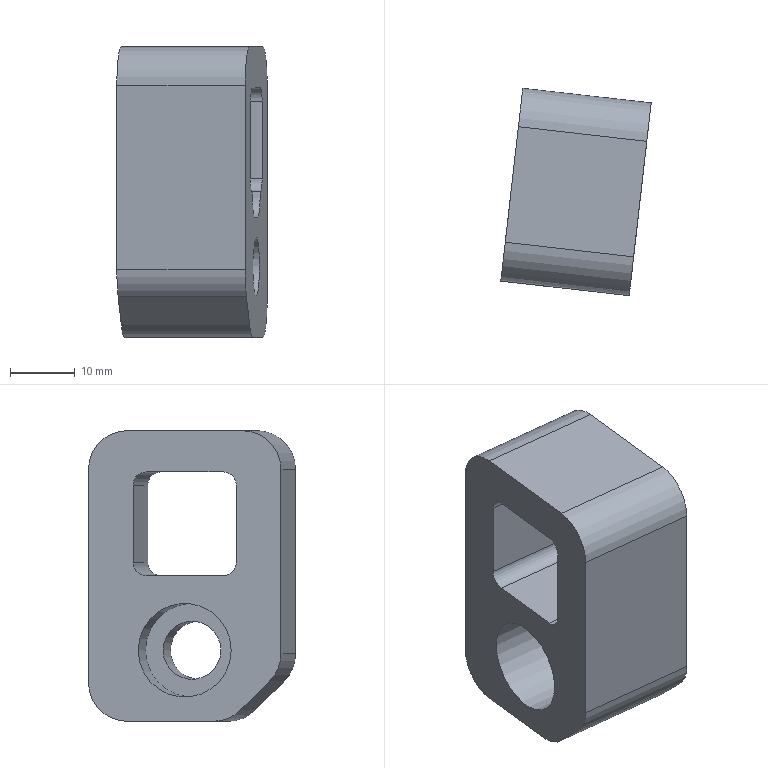Part | NX | features XQ 2 | 1 solid | 30 faces | box 23.268 x 32.071 x 45 mm | volume 18172 mm3 | plane 16 | cylinder 14 | commonest cylinder face diameters 12 x5 4.08 x4 8 x2 4 x1 9 x1 14.5 x1
STEP:
#1=CARTESIAN_POINT('',(3256.98,-253.634,-80.392));
#2=VERTEX_POINT('',#1);
#3=CARTESIAN_POINT('',(3257.49,-249.163,-80.392));
#4=DIRECTION('',(0.9936,-0.1132,0.));
#5=DIRECTION('',(-0.1132,-0.9936,0.));
#6=AXIS2_PLACEMENT_3D('',#3,#4,#5);
#7=CIRCLE('',#6,4.5);
#8=EDGE_CURVE('',#2,#2,#7,.T.);
#9=ORIENTED_EDGE('',*,*,#8,.F.);
#10=EDGE_LOOP('',(#9));
#11=FACE_BOUND('',#10,.T.);
#12=CARTESIAN_POINT('',(3259.188,-234.259,-85.392));
#13=VERTEX_POINT('',#12);
#14=CARTESIAN_POINT('',(3259.188,-234.259,-52.392));
#15=VERTEX_POINT('',#14);
#16=CARTESIAN_POINT('',(3259.188,-234.259,-78.616));
#17=DIRECTION('',(0.,0.,1.));
#18=VECTOR('',#17,1000.);
#19=LINE('',#16,#18);
#20=EDGE_CURVE('',#13,#15,#19,.T.);
#21=ORIENTED_EDGE('',*,*,#20,.T.);
#22=CARTESIAN_POINT('',(3258.508,-240.221,-46.392));
#23=VERTEX_POINT('',#22);
#24=CARTESIAN_POINT('',(3258.508,-240.221,-52.392));
#25=DIRECTION('',(0.9936,-0.1132,0.));
#26=DIRECTION('',(-0.1132,-0.9936,0.));
#27=AXIS2_PLACEMENT_3D('',#24,#25,#26);
#28=CIRCLE('',#27,6.);
#29=EDGE_CURVE('',#15,#23,#28,.T.);
#30=ORIENTED_EDGE('',*,*,#29,.T.);
#31=CARTESIAN_POINT('',(3256.471,-258.105,-46.392));
#32=VERTEX_POINT('',#31);
#33=CARTESIAN_POINT('',(3266.041,-174.108,-46.392));
#34=DIRECTION('',(-0.1132,-0.9936,0.));
#35=VECTOR('',#34,1000.);
#36=LINE('',#33,#35);
#37=EDGE_CURVE('',#23,#32,#36,.T.);
#38=ORIENTED_EDGE('',*,*,#37,.T.);
#39=CARTESIAN_POINT('',(3255.792,-264.066,-52.392));
#40=VERTEX_POINT('',#39);
#41=CARTESIAN_POINT('',(3256.471,-258.105,-52.392));
#42=DIRECTION('',(0.9936,-0.1132,0.));
#43=DIRECTION('',(-0.1132,-0.9936,0.));
#44=AXIS2_PLACEMENT_3D('',#41,#42,#43);
#45=CIRCLE('',#44,6.);
#46=EDGE_CURVE('',#32,#40,#45,.T.);
#47=ORIENTED_EDGE('',*,*,#46,.T.);
#48=CARTESIAN_POINT('',(3255.792,-264.066,-80.907));
#49=VERTEX_POINT('',#48);
#50=CARTESIAN_POINT('',(3255.792,-264.066,-78.616));
#51=DIRECTION('',(0.,0.,-1.));
#52=VECTOR('',#51,1000.);
#53=LINE('',#50,#52);
#54=EDGE_CURVE('',#40,#49,#53,.T.);
#55=ORIENTED_EDGE('',*,*,#54,.T.);
#56=CARTESIAN_POINT('',(3255.991,-262.32,-85.149));
#57=VERTEX_POINT('',#56);
#58=CARTESIAN_POINT('',(3256.471,-258.105,-80.907));
#59=DIRECTION('',(0.9936,-0.1132,0.));
#60=DIRECTION('',(-0.1132,-0.9936,0.));
#61=AXIS2_PLACEMENT_3D('',#58,#59,#60);
#62=CIRCLE('',#61,6.);
#63=EDGE_CURVE('',#49,#57,#62,.T.);
#64=ORIENTED_EDGE('',*,*,#63,.T.);
#65=CARTESIAN_POINT('',(3256.498,-257.864,-89.635));
#66=VERTEX_POINT('',#65);
#67=CARTESIAN_POINT('',(3260.646,-221.46,-126.274));
#68=DIRECTION('',(0.08005,0.7026,-0.7071));
#69=VECTOR('',#68,1000.);
#70=LINE('',#67,#69);
#71=EDGE_CURVE('',#57,#66,#70,.T.);
#72=ORIENTED_EDGE('',*,*,#71,.T.);
#73=CARTESIAN_POINT('',(3256.979,-253.648,-91.392));
#74=VERTEX_POINT('',#73);
#75=CARTESIAN_POINT('',(3256.979,-253.648,-85.392));
#76=DIRECTION('',(0.9936,-0.1132,0.));
#77=DIRECTION('',(-0.1132,-0.9936,0.));
#78=AXIS2_PLACEMENT_3D('',#75,#76,#77);
#79=CIRCLE('',#78,6.);
#80=EDGE_CURVE('',#66,#74,#79,.T.);
#81=ORIENTED_EDGE('',*,*,#80,.T.);
#82=CARTESIAN_POINT('',(3258.508,-240.221,-91.392));
#83=VERTEX_POINT('',#82);
#84=CARTESIAN_POINT('',(3266.041,-174.108,-91.392));
#85=DIRECTION('',(0.1132,0.9936,0.));
#86=VECTOR('',#85,1000.);
#87=LINE('',#84,#86);
#88=EDGE_CURVE('',#74,#83,#87,.T.);
#89=ORIENTED_EDGE('',*,*,#88,.T.);
#90=CARTESIAN_POINT('',(3258.508,-240.221,-85.392));
#91=DIRECTION('',(0.9936,-0.1132,0.));
#92=DIRECTION('',(-0.1132,-0.9936,0.));
#93=AXIS2_PLACEMENT_3D('',#90,#91,#92);
#94=CIRCLE('',#93,6.);
#95=EDGE_CURVE('',#83,#13,#94,.T.);
#96=ORIENTED_EDGE('',*,*,#95,.T.);
#97=EDGE_LOOP('',(#21,#30,#38,#47,#55,#64,#72,#81,#89,#96));
#98=FACE_BOUND('',#97,.T.);
#99=CARTESIAN_POINT('',(3257.32,-250.653,-72.892));
#100=VERTEX_POINT('',#99);
#101=CARTESIAN_POINT('',(3256.867,-254.627,-68.857));
#102=VERTEX_POINT('',#101);
#103=CARTESIAN_POINT('',(3257.32,-250.653,-68.892));
#104=DIRECTION('',(-0.9936,0.1132,0.));
#105=DIRECTION('',(-0.1132,-0.9936,0.));
#106=AXIS2_PLACEMENT_3D('',#103,#104,#105);
#107=CIRCLE('',#106,4.);
#108=EDGE_CURVE('',#100,#102,#107,.T.);
#109=ORIENTED_EDGE('',*,*,#108,.T.);
#110=CARTESIAN_POINT('',(3256.81,-255.124,-68.857));
#111=VERTEX_POINT('',#110);
#112=CARTESIAN_POINT('',(3258.112,-243.698,-68.857));
#113=DIRECTION('',(-0.1132,-0.9936,0.));
#114=VECTOR('',#113,1000.);
#115=LINE('',#112,#114);
#116=EDGE_CURVE('',#102,#111,#115,.T.);
#117=ORIENTED_EDGE('',*,*,#116,.T.);
#118=CARTESIAN_POINT('',(3256.579,-257.151,-66.817));
#119=VERTEX_POINT('',#118);
#120=CARTESIAN_POINT('',(3256.81,-255.124,-66.817));
#121=DIRECTION('',(-0.9936,0.1132,0.));
#122=DIRECTION('',(-0.1132,-0.9936,0.));
#123=AXIS2_PLACEMENT_3D('',#120,#121,#122);
#124=CIRCLE('',#123,2.04);
#125=EDGE_CURVE('',#111,#119,#124,.T.);
#126=ORIENTED_EDGE('',*,*,#125,.T.);
#127=CARTESIAN_POINT('',(3256.579,-257.151,-54.817));
#128=VERTEX_POINT('',#127);
#129=CARTESIAN_POINT('',(3256.579,-257.151,-66.817));
#130=DIRECTION('',(0.,-0.000000001,1.));
#131=VECTOR('',#130,1000.);
#132=LINE('',#129,#131);
#133=EDGE_CURVE('',#119,#128,#132,.T.);
#134=ORIENTED_EDGE('',*,*,#133,.T.);
#135=CARTESIAN_POINT('',(3256.81,-255.124,-52.777));
#136=VERTEX_POINT('',#135);
#137=CARTESIAN_POINT('',(3256.81,-255.124,-54.817));
#138=DIRECTION('',(-0.9936,0.1132,0.));
#139=DIRECTION('',(-0.1132,-0.9936,0.));
#140=AXIS2_PLACEMENT_3D('',#137,#138,#139);
#141=CIRCLE('',#140,2.04);
#142=EDGE_CURVE('',#128,#136,#141,.T.);
#143=ORIENTED_EDGE('',*,*,#142,.T.);
#144=CARTESIAN_POINT('',(3258.169,-243.201,-52.777));
#145=VERTEX_POINT('',#144);
#146=CARTESIAN_POINT('',(3256.81,-255.124,-52.777));
#147=DIRECTION('',(0.1132,0.9936,0.000000001));
#148=VECTOR('',#147,1000.);
#149=LINE('',#146,#148);
#150=EDGE_CURVE('',#136,#145,#149,.T.);
#151=ORIENTED_EDGE('',*,*,#150,.T.);
#152=CARTESIAN_POINT('',(3258.4,-241.174,-54.817));
#153=VERTEX_POINT('',#152);
#154=CARTESIAN_POINT('',(3258.169,-243.201,-54.817));
#155=DIRECTION('',(-0.9936,0.1132,0.));
#156=DIRECTION('',(-0.1132,-0.9936,0.));
#157=AXIS2_PLACEMENT_3D('',#154,#155,#156);
#158=CIRCLE('',#157,2.04);
#159=EDGE_CURVE('',#145,#153,#158,.T.);
#160=ORIENTED_EDGE('',*,*,#159,.T.);
#161=CARTESIAN_POINT('',(3258.4,-241.174,-66.817));
#162=VERTEX_POINT('',#161);
#163=CARTESIAN_POINT('',(3258.4,-241.174,-54.817));
#164=DIRECTION('',(0.,0.000000001,-1.));
#165=VECTOR('',#164,1000.);
#166=LINE('',#163,#165);
#167=EDGE_CURVE('',#153,#162,#166,.T.);
#168=ORIENTED_EDGE('',*,*,#167,.T.);
#169=CARTESIAN_POINT('',(3258.169,-243.201,-68.857));
#170=VERTEX_POINT('',#169);
#171=CARTESIAN_POINT('',(3258.169,-243.201,-66.817));
#172=DIRECTION('',(-0.9936,0.1132,0.));
#173=DIRECTION('',(-0.1132,-0.9936,0.));
#174=AXIS2_PLACEMENT_3D('',#171,#172,#173);
#175=CIRCLE('',#174,2.04);
#176=EDGE_CURVE('',#162,#170,#175,.T.);
#177=ORIENTED_EDGE('',*,*,#176,.T.);
#178=CARTESIAN_POINT('',(3258.112,-243.698,-68.857));
#179=VERTEX_POINT('',#178);
#180=CARTESIAN_POINT('',(3258.112,-243.698,-68.857));
#181=DIRECTION('',(-0.1132,-0.9936,0.));
#182=VECTOR('',#181,1000.);
#183=LINE('',#180,#182);
#184=EDGE_CURVE('',#170,#179,#183,.T.);
#185=ORIENTED_EDGE('',*,*,#184,.T.);
#186=CARTESIAN_POINT('',(3257.659,-247.672,-72.892));
#187=VERTEX_POINT('',#186);
#188=CARTESIAN_POINT('',(3257.659,-247.672,-68.892));
#189=DIRECTION('',(-0.9936,0.1132,0.));
#190=DIRECTION('',(-0.1132,-0.9936,0.));
#191=AXIS2_PLACEMENT_3D('',#188,#189,#190);
#192=CIRCLE('',#191,4.);
#193=EDGE_CURVE('',#179,#187,#192,.T.);
#194=ORIENTED_EDGE('',*,*,#193,.T.);
#195=CARTESIAN_POINT('',(3258.112,-243.698,-72.892));
#196=DIRECTION('',(-0.1132,-0.9936,0.));
#197=VECTOR('',#196,1000.);
#198=LINE('',#195,#197);
#199=EDGE_CURVE('',#187,#100,#198,.T.);
#200=ORIENTED_EDGE('',*,*,#199,.T.);
#201=EDGE_LOOP('',(#109,#117,#126,#134,#143,#151,#160,#168,#177,#185,#194,#200));
#202=FACE_BOUND('',#201,.T.);
#203=CARTESIAN_POINT('',(3266.041,-174.108,-78.616));
#204=DIRECTION('',(0.9936,-0.1132,0.));
#205=DIRECTION('',(-0.1132,-0.9936,0.));
#206=AXIS2_PLACEMENT_3D('',#203,#204,#205);
#207=PLANE('',#206);
#208=ADVANCED_FACE('',(#11,#98,#202),#207,.T.);
#209=CARTESIAN_POINT('',(3236.708,-254.887,-66.817));
#210=VERTEX_POINT('',#209);
#211=CARTESIAN_POINT('',(3236.708,-254.887,-54.817));
#212=VERTEX_POINT('',#211);
#213=CARTESIAN_POINT('',(3236.708,-254.887,-39.152));
#214=DIRECTION('',(0.,-0.000000001,1.));
#215=VECTOR('',#214,1000.);
#216=LINE('',#213,#215);
#217=EDGE_CURVE('',#210,#212,#216,.T.);
#218=ORIENTED_EDGE('',*,*,#217,.F.);
#219=CARTESIAN_POINT('',(3236.939,-252.86,-68.857));
#220=VERTEX_POINT('',#219);
#221=CARTESIAN_POINT('',(3236.939,-252.86,-66.817));
#222=DIRECTION('',(-0.9936,0.1132,0.));
#223=DIRECTION('',(0.1132,0.9936,0.));
#224=AXIS2_PLACEMENT_3D('',#221,#222,#223);
#225=CIRCLE('',#224,2.04);
#226=EDGE_CURVE('',#220,#210,#225,.T.);
#227=ORIENTED_EDGE('',*,*,#226,.F.);
#228=CARTESIAN_POINT('',(3238.297,-240.937,-68.857));
#229=VERTEX_POINT('',#228);
#230=CARTESIAN_POINT('',(3256.924,-77.454,-68.857));
#231=DIRECTION('',(-0.1132,-0.9936,0.));
#232=VECTOR('',#231,1000.);
#233=LINE('',#230,#232);
#234=EDGE_CURVE('',#229,#220,#233,.T.);
#235=ORIENTED_EDGE('',*,*,#234,.F.);
#236=CARTESIAN_POINT('',(3238.528,-238.91,-66.817));
#237=VERTEX_POINT('',#236);
#238=CARTESIAN_POINT('',(3238.297,-240.937,-66.817));
#239=DIRECTION('',(-0.9936,0.1132,0.));
#240=DIRECTION('',(0.1132,0.9936,0.));
#241=AXIS2_PLACEMENT_3D('',#238,#239,#240);
#242=CIRCLE('',#241,2.04);
#243=EDGE_CURVE('',#237,#229,#242,.T.);
#244=ORIENTED_EDGE('',*,*,#243,.F.);
#245=CARTESIAN_POINT('',(3238.528,-238.91,-54.817));
#246=VERTEX_POINT('',#245);
#247=CARTESIAN_POINT('',(3238.528,-238.91,-39.152));
#248=DIRECTION('',(0.,0.000000001,-1.));
#249=VECTOR('',#248,1000.);
#250=LINE('',#247,#249);
#251=EDGE_CURVE('',#246,#237,#250,.T.);
#252=ORIENTED_EDGE('',*,*,#251,.F.);
#253=CARTESIAN_POINT('',(3238.297,-240.937,-52.777));
#254=VERTEX_POINT('',#253);
#255=CARTESIAN_POINT('',(3238.297,-240.937,-54.817));
#256=DIRECTION('',(-0.9936,0.1132,0.));
#257=DIRECTION('',(0.1132,0.9936,0.));
#258=AXIS2_PLACEMENT_3D('',#255,#256,#257);
#259=CIRCLE('',#258,2.04);
#260=EDGE_CURVE('',#254,#246,#259,.T.);
#261=ORIENTED_EDGE('',*,*,#260,.F.);
#262=CARTESIAN_POINT('',(3236.939,-252.86,-52.777));
#263=VERTEX_POINT('',#262);
#264=CARTESIAN_POINT('',(3256.924,-77.454,-52.777));
#265=DIRECTION('',(0.1132,0.9936,0.000000001));
#266=VECTOR('',#265,1000.);
#267=LINE('',#264,#266);
#268=EDGE_CURVE('',#263,#254,#267,.T.);
#269=ORIENTED_EDGE('',*,*,#268,.F.);
#270=CARTESIAN_POINT('',(3236.939,-252.86,-54.817));
#271=DIRECTION('',(-0.9936,0.1132,0.));
#272=DIRECTION('',(0.1132,0.9936,0.));
#273=AXIS2_PLACEMENT_3D('',#270,#271,#272);
#274=CIRCLE('',#273,2.04);
#275=EDGE_CURVE('',#212,#263,#274,.T.);
#276=ORIENTED_EDGE('',*,*,#275,.F.);
#277=EDGE_LOOP('',(#218,#227,#235,#244,#252,#261,#269,#276));
#278=FACE_BOUND('',#277,.T.);
#279=CARTESIAN_POINT('',(3236.599,-255.841,-46.392));
#280=VERTEX_POINT('',#279);
#281=CARTESIAN_POINT('',(3238.637,-237.957,-46.392));
#282=VERTEX_POINT('',#281);
#283=CARTESIAN_POINT('',(3256.924,-77.454,-46.392));
#284=DIRECTION('',(0.1132,0.9936,0.));
#285=VECTOR('',#284,1000.);
#286=LINE('',#283,#285);
#287=EDGE_CURVE('',#280,#282,#286,.T.);
#288=ORIENTED_EDGE('',*,*,#287,.T.);
#289=CARTESIAN_POINT('',(3239.316,-231.995,-52.392));
#290=VERTEX_POINT('',#289);
#291=CARTESIAN_POINT('',(3238.637,-237.957,-52.392));
#292=DIRECTION('',(-0.9936,0.1132,0.));
#293=DIRECTION('',(0.1132,0.9936,0.));
#294=AXIS2_PLACEMENT_3D('',#291,#292,#293);
#295=CIRCLE('',#294,6.);
#296=EDGE_CURVE('',#282,#290,#295,.T.);
#297=ORIENTED_EDGE('',*,*,#296,.T.);
#298=CARTESIAN_POINT('',(3239.316,-231.995,-85.392));
#299=VERTEX_POINT('',#298);
#300=CARTESIAN_POINT('',(3239.316,-231.995,-39.152));
#301=DIRECTION('',(0.,0.,-1.));
#302=VECTOR('',#301,1000.);
#303=LINE('',#300,#302);
#304=EDGE_CURVE('',#290,#299,#303,.T.);
#305=ORIENTED_EDGE('',*,*,#304,.T.);
#306=CARTESIAN_POINT('',(3238.637,-237.957,-91.392));
#307=VERTEX_POINT('',#306);
#308=CARTESIAN_POINT('',(3238.637,-237.957,-85.392));
#309=DIRECTION('',(-0.9936,0.1132,0.));
#310=DIRECTION('',(0.1132,0.9936,0.));
#311=AXIS2_PLACEMENT_3D('',#308,#309,#310);
#312=CIRCLE('',#311,6.);
#313=EDGE_CURVE('',#299,#307,#312,.T.);
#314=ORIENTED_EDGE('',*,*,#313,.T.);
#315=CARTESIAN_POINT('',(3237.107,-251.384,-91.392));
#316=VERTEX_POINT('',#315);
#317=CARTESIAN_POINT('',(3256.924,-77.454,-91.392));
#318=DIRECTION('',(-0.1132,-0.9936,0.));
#319=VECTOR('',#318,1000.);
#320=LINE('',#317,#319);
#321=EDGE_CURVE('',#307,#316,#320,.T.);
#322=ORIENTED_EDGE('',*,*,#321,.T.);
#323=CARTESIAN_POINT('',(3236.627,-255.6,-89.635));
#324=VERTEX_POINT('',#323);
#325=CARTESIAN_POINT('',(3237.107,-251.384,-85.392));
#326=DIRECTION('',(-0.9936,0.1132,0.));
#327=DIRECTION('',(0.1132,0.9936,0.));
#328=AXIS2_PLACEMENT_3D('',#325,#326,#327);
#329=CIRCLE('',#328,6.);
#330=EDGE_CURVE('',#316,#324,#329,.T.);
#331=ORIENTED_EDGE('',*,*,#330,.T.);
#332=CARTESIAN_POINT('',(3236.119,-260.056,-85.149));
#333=VERTEX_POINT('',#332);
#334=CARTESIAN_POINT('',(3243.918,-191.606,-154.042));
#335=DIRECTION('',(-0.08005,-0.7026,0.7071));
#336=VECTOR('',#335,1000.);
#337=LINE('',#334,#336);
#338=EDGE_CURVE('',#324,#333,#337,.T.);
#339=ORIENTED_EDGE('',*,*,#338,.T.);
#340=CARTESIAN_POINT('',(3235.92,-261.802,-80.907));
#341=VERTEX_POINT('',#340);
#342=CARTESIAN_POINT('',(3236.599,-255.841,-80.907));
#343=DIRECTION('',(-0.9936,0.1132,0.));
#344=DIRECTION('',(0.1132,0.9936,0.));
#345=AXIS2_PLACEMENT_3D('',#342,#343,#344);
#346=CIRCLE('',#345,6.);
#347=EDGE_CURVE('',#333,#341,#346,.T.);
#348=ORIENTED_EDGE('',*,*,#347,.T.);
#349=CARTESIAN_POINT('',(3235.92,-261.802,-52.392));
#350=VERTEX_POINT('',#349);
#351=CARTESIAN_POINT('',(3235.92,-261.802,-39.152));
#352=DIRECTION('',(0.,0.,1.));
#353=VECTOR('',#352,1000.);
#354=LINE('',#351,#353);
#355=EDGE_CURVE('',#341,#350,#354,.T.);
#356=ORIENTED_EDGE('',*,*,#355,.T.);
#357=CARTESIAN_POINT('',(3236.599,-255.841,-52.392));
#358=DIRECTION('',(-0.9936,0.1132,0.));
#359=DIRECTION('',(0.1132,0.9936,0.));
#360=AXIS2_PLACEMENT_3D('',#357,#358,#359);
#361=CIRCLE('',#360,6.);
#362=EDGE_CURVE('',#350,#280,#361,.T.);
#363=ORIENTED_EDGE('',*,*,#362,.T.);
#364=EDGE_LOOP('',(#288,#297,#305,#314,#322,#331,#339,#348,#356,#363));
#365=FACE_BOUND('',#364,.T.);
#366=CARTESIAN_POINT('',(3238.439,-239.695,-80.392));
#367=VERTEX_POINT('',#366);
#368=CARTESIAN_POINT('',(3237.618,-246.899,-80.392));
#369=DIRECTION('',(0.9936,-0.1132,0.));
#370=DIRECTION('',(0.1132,0.9936,0.));
#371=AXIS2_PLACEMENT_3D('',#368,#369,#370);
#372=CIRCLE('',#371,7.25);
#373=EDGE_CURVE('',#367,#367,#372,.T.);
#374=ORIENTED_EDGE('',*,*,#373,.T.);
#375=EDGE_LOOP('',(#374));
#376=FACE_BOUND('',#375,.T.);
#377=CARTESIAN_POINT('',(3256.924,-77.454,-39.152));
#378=DIRECTION('',(-0.9936,0.1132,0.));
#379=DIRECTION('',(0.,0.,-1.));
#380=AXIS2_PLACEMENT_3D('',#377,#378,#379);
#381=PLANE('',#380);
#382=ADVANCED_FACE('',(#278,#365,#376),#381,.T.);
#383=ORIENTED_EDGE('',*,*,#37,.F.);
#384=CARTESIAN_POINT('',(3233.669,-237.391,-46.392));
#385=DIRECTION('',(-0.9936,0.1132,0.));
#386=VECTOR('',#385,1000.);
#387=LINE('',#384,#386);
#388=EDGE_CURVE('',#23,#282,#387,.T.);
#389=ORIENTED_EDGE('',*,*,#388,.T.);
#390=ORIENTED_EDGE('',*,*,#287,.F.);
#391=CARTESIAN_POINT('',(3231.631,-255.275,-46.392));
#392=DIRECTION('',(0.9936,-0.1132,0.));
#393=VECTOR('',#392,1000.);
#394=LINE('',#391,#393);
#395=EDGE_CURVE('',#280,#32,#394,.T.);
#396=ORIENTED_EDGE('',*,*,#395,.T.);
#397=EDGE_LOOP('',(#383,#389,#390,#396));
#398=FACE_BOUND('',#397,.T.);
#399=CARTESIAN_POINT('',(3232.65,-246.333,-46.392));
#400=DIRECTION('',(0.,0.,1.));
#401=DIRECTION('',(-0.9981,-0.06105,0.));
#402=AXIS2_PLACEMENT_3D('',#399,#400,#401);
#403=PLANE('',#402);
#404=ADVANCED_FACE('',(#398),#403,.T.);
#405=ORIENTED_EDGE('',*,*,#304,.F.);
#406=CARTESIAN_POINT('',(3234.348,-231.429,-52.392));
#407=DIRECTION('',(0.9936,-0.1132,0.));
#408=VECTOR('',#407,1000.);
#409=LINE('',#406,#408);
#410=EDGE_CURVE('',#290,#15,#409,.T.);
#411=ORIENTED_EDGE('',*,*,#410,.T.);
#412=ORIENTED_EDGE('',*,*,#20,.F.);
#413=CARTESIAN_POINT('',(3234.348,-231.429,-85.392));
#414=DIRECTION('',(-0.9936,0.1132,0.));
#415=VECTOR('',#414,1000.);
#416=LINE('',#413,#415);
#417=EDGE_CURVE('',#13,#299,#416,.T.);
#418=ORIENTED_EDGE('',*,*,#417,.T.);
#419=EDGE_LOOP('',(#405,#411,#412,#418));
#420=FACE_BOUND('',#419,.T.);
#421=CARTESIAN_POINT('',(3234.348,-231.429,-60.817));
#422=DIRECTION('',(0.1132,0.9936,0.));
#423=DIRECTION('',(0.9936,-0.1132,0.));
#424=AXIS2_PLACEMENT_3D('',#421,#422,#423);
#425=PLANE('',#424);
#426=ADVANCED_FACE('',(#420),#425,.T.);
#427=ORIENTED_EDGE('',*,*,#54,.F.);
#428=CARTESIAN_POINT('',(3230.952,-261.236,-52.392));
#429=DIRECTION('',(-0.9936,0.1132,0.));
#430=VECTOR('',#429,1000.);
#431=LINE('',#428,#430);
#432=EDGE_CURVE('',#40,#350,#431,.T.);
#433=ORIENTED_EDGE('',*,*,#432,.T.);
#434=ORIENTED_EDGE('',*,*,#355,.F.);
#435=CARTESIAN_POINT('',(3230.952,-261.236,-80.907));
#436=DIRECTION('',(0.9936,-0.1132,0.));
#437=VECTOR('',#436,1000.);
#438=LINE('',#435,#437);
#439=EDGE_CURVE('',#341,#49,#438,.T.);
#440=ORIENTED_EDGE('',*,*,#439,.T.);
#441=EDGE_LOOP('',(#427,#433,#434,#440));
#442=FACE_BOUND('',#441,.T.);
#443=CARTESIAN_POINT('',(3230.952,-261.236,-60.817));
#444=DIRECTION('',(-0.1132,-0.9936,0.));
#445=DIRECTION('',(-0.9936,0.1132,0.));
#446=AXIS2_PLACEMENT_3D('',#443,#444,#445);
#447=PLANE('',#446);
#448=ADVANCED_FACE('',(#442),#447,.T.);
#449=ORIENTED_EDGE('',*,*,#88,.F.);
#450=CARTESIAN_POINT('',(3232.139,-250.818,-91.392));
#451=DIRECTION('',(-0.9936,0.1132,0.));
#452=VECTOR('',#451,1000.);
#453=LINE('',#450,#452);
#454=EDGE_CURVE('',#74,#316,#453,.T.);
#455=ORIENTED_EDGE('',*,*,#454,.T.);
#456=ORIENTED_EDGE('',*,*,#321,.F.);
#457=CARTESIAN_POINT('',(3233.669,-237.391,-91.392));
#458=DIRECTION('',(0.9936,-0.1132,0.));
#459=VECTOR('',#458,1000.);
#460=LINE('',#457,#459);
#461=EDGE_CURVE('',#307,#83,#460,.T.);
#462=ORIENTED_EDGE('',*,*,#461,.T.);
#463=EDGE_LOOP('',(#449,#455,#456,#462));
#464=FACE_BOUND('',#463,.T.);
#465=CARTESIAN_POINT('',(3232.65,-246.333,-91.392));
#466=DIRECTION('',(0.,0.,-1.));
#467=DIRECTION('',(0.9981,0.06105,0.));
#468=AXIS2_PLACEMENT_3D('',#465,#466,#467);
#469=PLANE('',#468);
#470=ADVANCED_FACE('',(#464),#469,.T.);
#471=ORIENTED_EDGE('',*,*,#71,.F.);
#472=CARTESIAN_POINT('',(3231.151,-259.49,-85.149));
#473=DIRECTION('',(-0.9936,0.1132,0.));
#474=VECTOR('',#473,1000.);
#475=LINE('',#472,#474);
#476=EDGE_CURVE('',#57,#333,#475,.T.);
#477=ORIENTED_EDGE('',*,*,#476,.T.);
#478=ORIENTED_EDGE('',*,*,#338,.F.);
#479=CARTESIAN_POINT('',(3231.659,-255.034,-89.635));
#480=DIRECTION('',(0.9936,-0.1132,0.));
#481=VECTOR('',#480,1000.);
#482=LINE('',#479,#481);
#483=EDGE_CURVE('',#324,#66,#482,.T.);
#484=ORIENTED_EDGE('',*,*,#483,.T.);
#485=EDGE_LOOP('',(#471,#477,#478,#484));
#486=FACE_BOUND('',#485,.T.);
#487=CARTESIAN_POINT('',(3231.179,-259.249,-85.392));
#488=DIRECTION('',(0.08005,0.7026,0.7071));
#489=DIRECTION('',(0.9936,-0.1132,0.));
#490=AXIS2_PLACEMENT_3D('',#487,#488,#489);
#491=PLANE('',#490);
#492=ADVANCED_FACE('',(#486),#491,.F.);
#493=ORIENTED_EDGE('',*,*,#296,.F.);
#494=ORIENTED_EDGE('',*,*,#388,.F.);
#495=ORIENTED_EDGE('',*,*,#29,.F.);
#496=ORIENTED_EDGE('',*,*,#410,.F.);
#497=EDGE_LOOP('',(#493,#494,#495,#496));
#498=FACE_BOUND('',#497,.T.);
#499=CARTESIAN_POINT('',(3233.669,-237.391,-52.392));
#500=DIRECTION('',(0.9936,-0.1132,0.));
#501=DIRECTION('',(-0.1132,-0.9936,0.));
#502=AXIS2_PLACEMENT_3D('',#499,#500,#501);
#503=CYLINDRICAL_SURFACE('',#502,6.);
#504=ADVANCED_FACE('',(#498),#503,.T.);
#505=ORIENTED_EDGE('',*,*,#46,.F.);
#506=ORIENTED_EDGE('',*,*,#395,.F.);
#507=ORIENTED_EDGE('',*,*,#362,.F.);
#508=ORIENTED_EDGE('',*,*,#432,.F.);
#509=EDGE_LOOP('',(#505,#506,#507,#508));
#510=FACE_BOUND('',#509,.T.);
#511=CARTESIAN_POINT('',(3231.631,-255.275,-52.392));
#512=DIRECTION('',(-0.9936,0.1132,0.));
#513=DIRECTION('',(0.1132,0.9936,0.));
#514=AXIS2_PLACEMENT_3D('',#511,#512,#513);
#515=CYLINDRICAL_SURFACE('',#514,6.);
#516=ADVANCED_FACE('',(#510),#515,.T.);
#517=ORIENTED_EDGE('',*,*,#347,.F.);
#518=ORIENTED_EDGE('',*,*,#476,.F.);
#519=ORIENTED_EDGE('',*,*,#63,.F.);
#520=ORIENTED_EDGE('',*,*,#439,.F.);
#521=EDGE_LOOP('',(#517,#518,#519,#520));
#522=FACE_BOUND('',#521,.T.);
#523=CARTESIAN_POINT('',(3231.631,-255.275,-80.907));
#524=DIRECTION('',(-0.9936,0.1132,0.));
#525=DIRECTION('',(0.1132,0.9936,0.));
#526=AXIS2_PLACEMENT_3D('',#523,#524,#525);
#527=CYLINDRICAL_SURFACE('',#526,6.);
#528=ADVANCED_FACE('',(#522),#527,.T.);
#529=ORIENTED_EDGE('',*,*,#80,.F.);
#530=ORIENTED_EDGE('',*,*,#483,.F.);
#531=ORIENTED_EDGE('',*,*,#330,.F.);
#532=ORIENTED_EDGE('',*,*,#454,.F.);
#533=EDGE_LOOP('',(#529,#530,#531,#532));
#534=FACE_BOUND('',#533,.T.);
#535=CARTESIAN_POINT('',(3232.139,-250.818,-85.392));
#536=DIRECTION('',(0.9936,-0.1132,0.));
#537=DIRECTION('',(-0.1132,-0.9936,0.));
#538=AXIS2_PLACEMENT_3D('',#535,#536,#537);
#539=CYLINDRICAL_SURFACE('',#538,6.);
#540=ADVANCED_FACE('',(#534),#539,.T.);
#541=ORIENTED_EDGE('',*,*,#313,.F.);
#542=ORIENTED_EDGE('',*,*,#417,.F.);
#543=ORIENTED_EDGE('',*,*,#95,.F.);
#544=ORIENTED_EDGE('',*,*,#461,.F.);
#545=EDGE_LOOP('',(#541,#542,#543,#544));
#546=FACE_BOUND('',#545,.T.);
#547=CARTESIAN_POINT('',(3233.669,-237.391,-85.392));
#548=DIRECTION('',(0.9936,-0.1132,0.));
#549=DIRECTION('',(-0.1132,-0.9936,0.));
#550=AXIS2_PLACEMENT_3D('',#547,#548,#549);
#551=CYLINDRICAL_SURFACE('',#550,6.);
#552=ADVANCED_FACE('',(#546),#551,.T.);
#553=ORIENTED_EDGE('',*,*,#8,.T.);
#554=EDGE_LOOP('',(#553));
#555=FACE_BOUND('',#554,.T.);
#556=CARTESIAN_POINT('',(3247.044,-252.502,-80.392));
#557=VERTEX_POINT('',#556);
#558=CARTESIAN_POINT('',(3247.554,-248.031,-80.392));
#559=DIRECTION('',(0.9936,-0.1132,0.));
#560=DIRECTION('',(-0.1132,-0.9936,0.));
#561=AXIS2_PLACEMENT_3D('',#558,#559,#560);
#562=CIRCLE('',#561,4.5);
#563=EDGE_CURVE('',#557,#557,#562,.T.);
#564=ORIENTED_EDGE('',*,*,#563,.F.);
#565=EDGE_LOOP('',(#564));
#566=FACE_BOUND('',#565,.T.);
#567=CARTESIAN_POINT('',(3232.65,-246.333,-80.392));
#568=DIRECTION('',(0.9936,-0.1132,0.));
#569=DIRECTION('',(0.01966,0.1725,0.9848));
#570=AXIS2_PLACEMENT_3D('',#567,#568,#569);
#571=CYLINDRICAL_SURFACE('',#570,4.5);
#572=ADVANCED_FACE('',(#555,#566),#571,.F.);
#573=ORIENTED_EDGE('',*,*,#563,.T.);
#574=EDGE_LOOP('',(#573));
#575=FACE_BOUND('',#574,.T.);
#576=CARTESIAN_POINT('',(3246.733,-255.234,-80.392));
#577=VERTEX_POINT('',#576);
#578=CARTESIAN_POINT('',(3247.554,-248.031,-80.392));
#579=DIRECTION('',(0.9936,-0.1132,0.));
#580=DIRECTION('',(-0.1132,-0.9936,0.));
#581=AXIS2_PLACEMENT_3D('',#578,#579,#580);
#582=CIRCLE('',#581,7.25);
#583=EDGE_CURVE('',#577,#577,#582,.T.);
#584=ORIENTED_EDGE('',*,*,#583,.F.);
#585=EDGE_LOOP('',(#584));
#586=FACE_BOUND('',#585,.T.);
#587=CARTESIAN_POINT('',(3247.554,-248.031,-80.392));
#588=DIRECTION('',(0.9936,-0.1132,0.));
#589=DIRECTION('',(-0.1132,-0.9936,0.));
#590=AXIS2_PLACEMENT_3D('',#587,#588,#589);
#591=PLANE('',#590);
#592=ADVANCED_FACE('',(#575,#586),#591,.F.);
#593=ORIENTED_EDGE('',*,*,#583,.T.);
#594=EDGE_LOOP('',(#593));
#595=FACE_BOUND('',#594,.T.);
#596=ORIENTED_EDGE('',*,*,#373,.F.);
#597=EDGE_LOOP('',(#596));
#598=FACE_BOUND('',#597,.T.);
#599=CARTESIAN_POINT('',(3232.65,-246.333,-80.392));
#600=DIRECTION('',(0.9936,-0.1132,0.));
#601=DIRECTION('',(0.01966,0.1725,0.9848));
#602=AXIS2_PLACEMENT_3D('',#599,#600,#601);
#603=CYLINDRICAL_SURFACE('',#602,7.25);
#604=ADVANCED_FACE('',(#595,#598),#603,.F.);
#605=ORIENTED_EDGE('',*,*,#199,.F.);
#606=CARTESIAN_POINT('',(3249.711,-246.767,-72.892));
#607=VERTEX_POINT('',#606);
#608=CARTESIAN_POINT('',(3249.711,-246.767,-72.892));
#609=DIRECTION('',(-0.9936,0.1132,0.));
#610=VECTOR('',#609,1000.);
#611=LINE('',#608,#610);
#612=EDGE_CURVE('',#187,#607,#611,.T.);
#613=ORIENTED_EDGE('',*,*,#612,.T.);
#614=CARTESIAN_POINT('',(3249.371,-249.747,-72.892));
#615=VERTEX_POINT('',#614);
#616=CARTESIAN_POINT('',(3250.164,-242.792,-72.892));
#617=DIRECTION('',(-0.1132,-0.9936,0.));
#618=VECTOR('',#617,1000.);
#619=LINE('',#616,#618);
#620=EDGE_CURVE('',#607,#615,#619,.T.);
#621=ORIENTED_EDGE('',*,*,#620,.T.);
#622=CARTESIAN_POINT('',(3257.32,-250.653,-72.892));
#623=DIRECTION('',(0.9936,-0.1132,0.));
#624=VECTOR('',#623,1000.);
#625=LINE('',#622,#624);
#626=EDGE_CURVE('',#615,#100,#625,.T.);
#627=ORIENTED_EDGE('',*,*,#626,.T.);
#628=EDGE_LOOP('',(#605,#613,#621,#627));
#629=FACE_BOUND('',#628,.T.);
#630=CARTESIAN_POINT('',(3297.855,-248.226,-72.892));
#631=DIRECTION('',(0.,0.,-1.));
#632=DIRECTION('',(0.06105,-0.9981,0.));
#633=AXIS2_PLACEMENT_3D('',#630,#631,#632);
#634=PLANE('',#633);
#635=ADVANCED_FACE('',(#629),#634,.F.);
#636=CARTESIAN_POINT('',(3248.918,-253.722,-68.857));
#637=VERTEX_POINT('',#636);
#638=CARTESIAN_POINT('',(3249.145,-251.735,-68.857));
#639=VERTEX_POINT('',#638);
#640=CARTESIAN_POINT('',(3258.092,-173.202,-68.857));
#641=DIRECTION('',(0.1132,0.9936,0.));
#642=VECTOR('',#641,1000.);
#643=LINE('',#640,#642);
#644=EDGE_CURVE('',#637,#639,#643,.T.);
#645=ORIENTED_EDGE('',*,*,#644,.F.);
#646=CARTESIAN_POINT('',(3249.371,-249.747,-68.892));
#647=DIRECTION('',(0.9936,-0.1132,0.));
#648=DIRECTION('',(-0.1132,-0.9936,0.));
#649=AXIS2_PLACEMENT_3D('',#646,#647,#648);
#650=CIRCLE('',#649,4.);
#651=EDGE_CURVE('',#637,#615,#650,.T.);
#652=ORIENTED_EDGE('',*,*,#651,.T.);
#653=ORIENTED_EDGE('',*,*,#620,.F.);
#654=CARTESIAN_POINT('',(3250.164,-242.793,-68.857));
#655=VERTEX_POINT('',#654);
#656=CARTESIAN_POINT('',(3249.711,-246.767,-68.892));
#657=DIRECTION('',(0.9936,-0.1132,0.));
#658=DIRECTION('',(-0.1132,-0.9936,0.));
#659=AXIS2_PLACEMENT_3D('',#656,#657,#658);
#660=CIRCLE('',#659,4.);
#661=EDGE_CURVE('',#607,#655,#660,.T.);
#662=ORIENTED_EDGE('',*,*,#661,.T.);
#663=CARTESIAN_POINT('',(3249.937,-244.78,-68.857));
#664=VERTEX_POINT('',#663);
#665=CARTESIAN_POINT('',(3258.092,-173.202,-68.857));
#666=DIRECTION('',(0.1132,0.9936,0.));
#667=VECTOR('',#666,1000.);
#668=LINE('',#665,#667);
#669=EDGE_CURVE('',#664,#655,#668,.T.);
#670=ORIENTED_EDGE('',*,*,#669,.F.);
#671=CARTESIAN_POINT('',(3249.937,-244.78,-70.857));
#672=VERTEX_POINT('',#671);
#673=CARTESIAN_POINT('',(3249.937,-244.78,-78.616));
#674=DIRECTION('',(0.,0.,-1.));
#675=VECTOR('',#674,1000.);
#676=LINE('',#673,#675);
#677=EDGE_CURVE('',#664,#672,#676,.T.);
#678=ORIENTED_EDGE('',*,*,#677,.T.);
#679=CARTESIAN_POINT('',(3249.145,-251.735,-70.857));
#680=VERTEX_POINT('',#679);
#681=CARTESIAN_POINT('',(3250.164,-242.792,-70.857));
#682=DIRECTION('',(0.1132,0.9936,0.));
#683=VECTOR('',#682,1000.);
#684=LINE('',#681,#683);
#685=EDGE_CURVE('',#680,#672,#684,.T.);
#686=ORIENTED_EDGE('',*,*,#685,.F.);
#687=CARTESIAN_POINT('',(3249.145,-251.735,-78.616));
#688=DIRECTION('',(0.,0.,-1.));
#689=VECTOR('',#688,1000.);
#690=LINE('',#687,#689);
#691=EDGE_CURVE('',#639,#680,#690,.T.);
#692=ORIENTED_EDGE('',*,*,#691,.F.);
#693=EDGE_LOOP('',(#645,#652,#653,#662,#670,#678,#686,#692));
#694=FACE_BOUND('',#693,.T.);
#695=CARTESIAN_POINT('',(3258.092,-173.202,-78.616));
#696=DIRECTION('',(0.9936,-0.1132,0.));
#697=DIRECTION('',(-0.1132,-0.9936,0.));
#698=AXIS2_PLACEMENT_3D('',#695,#696,#697);
#699=PLANE('',#698);
#700=ADVANCED_FACE('',(#694),#699,.T.);
#701=ORIENTED_EDGE('',*,*,#193,.F.);
#702=CARTESIAN_POINT('',(3297.855,-248.226,-68.857));
#703=DIRECTION('',(-0.9936,0.1132,0.));
#704=VECTOR('',#703,1000.);
#705=LINE('',#702,#704);
#706=EDGE_CURVE('',#179,#655,#705,.T.);
#707=ORIENTED_EDGE('',*,*,#706,.T.);
#708=ORIENTED_EDGE('',*,*,#661,.F.);
#709=ORIENTED_EDGE('',*,*,#612,.F.);
#710=EDGE_LOOP('',(#701,#707,#708,#709));
#711=FACE_BOUND('',#710,.T.);
#712=CARTESIAN_POINT('',(3297.402,-252.201,-68.892));
#713=DIRECTION('',(0.9936,-0.1132,0.));
#714=DIRECTION('',(-0.1132,-0.9936,0.));
#715=AXIS2_PLACEMENT_3D('',#712,#713,#714);
#716=CYLINDRICAL_SURFACE('',#715,4.);
#717=ADVANCED_FACE('',(#711),#716,.F.);
#718=ORIENTED_EDGE('',*,*,#651,.F.);
#719=CARTESIAN_POINT('',(3296.61,-259.155,-68.857));
#720=DIRECTION('',(0.9936,-0.1132,0.));
#721=VECTOR('',#720,1000.);
#722=LINE('',#719,#721);
#723=EDGE_CURVE('',#637,#102,#722,.T.);
#724=ORIENTED_EDGE('',*,*,#723,.T.);
#725=ORIENTED_EDGE('',*,*,#108,.F.);
#726=ORIENTED_EDGE('',*,*,#626,.F.);
#727=EDGE_LOOP('',(#718,#724,#725,#726));
#728=FACE_BOUND('',#727,.T.);
#729=CARTESIAN_POINT('',(3297.063,-255.181,-68.892));
#730=DIRECTION('',(-0.9936,0.1132,0.));
#731=DIRECTION('',(0.1132,0.9936,0.));
#732=AXIS2_PLACEMENT_3D('',#729,#730,#731);
#733=CYLINDRICAL_SURFACE('',#732,4.);
#734=ADVANCED_FACE('',(#728),#733,.F.);
#735=ORIENTED_EDGE('',*,*,#217,.T.);
#736=CARTESIAN_POINT('',(3205.907,-251.378,-54.817));
#737=DIRECTION('',(0.9936,-0.1132,-0.000000001));
#738=VECTOR('',#737,1000.);
#739=LINE('',#736,#738);
#740=EDGE_CURVE('',#212,#128,#739,.T.);
#741=ORIENTED_EDGE('',*,*,#740,.T.);
#742=ORIENTED_EDGE('',*,*,#133,.F.);
#743=CARTESIAN_POINT('',(3296.322,-261.679,-66.817));
#744=DIRECTION('',(0.9936,-0.1132,0.));
#745=VECTOR('',#744,1000.);
#746=LINE('',#743,#745);
#747=EDGE_CURVE('',#210,#119,#746,.T.);
#748=ORIENTED_EDGE('',*,*,#747,.F.);
#749=EDGE_LOOP('',(#735,#741,#742,#748));
#750=FACE_BOUND('',#749,.T.);
#751=CARTESIAN_POINT('',(3205.907,-251.378,-66.817));
#752=DIRECTION('',(-0.1132,-0.9936,-0.000000001));
#753=DIRECTION('',(0.9936,-0.1132,0.));
#754=AXIS2_PLACEMENT_3D('',#751,#752,#753);
#755=PLANE('',#754);
#756=ADVANCED_FACE('',(#750),#755,.F.);
#757=ORIENTED_EDGE('',*,*,#275,.T.);
#758=CARTESIAN_POINT('',(3206.138,-249.351,-52.777));
#759=DIRECTION('',(0.9936,-0.1132,-0.000000001));
#760=VECTOR('',#759,1000.);
#761=LINE('',#758,#760);
#762=EDGE_CURVE('',#263,#136,#761,.T.);
#763=ORIENTED_EDGE('',*,*,#762,.T.);
#764=ORIENTED_EDGE('',*,*,#142,.F.);
#765=ORIENTED_EDGE('',*,*,#740,.F.);
#766=EDGE_LOOP('',(#757,#763,#764,#765));
#767=FACE_BOUND('',#766,.T.);
#768=CARTESIAN_POINT('',(3206.138,-249.351,-54.817));
#769=DIRECTION('',(-0.9936,0.1132,0.000000001));
#770=DIRECTION('',(-0.1132,-0.9936,0.));
#771=AXIS2_PLACEMENT_3D('',#768,#769,#770);
#772=CYLINDRICAL_SURFACE('',#771,2.04);
#773=ADVANCED_FACE('',(#767),#772,.F.);
#774=ORIENTED_EDGE('',*,*,#268,.T.);
#775=CARTESIAN_POINT('',(3207.497,-237.428,-52.777));
#776=DIRECTION('',(0.9936,-0.1132,-0.000000001));
#777=VECTOR('',#776,1000.);
#778=LINE('',#775,#777);
#779=EDGE_CURVE('',#254,#145,#778,.T.);
#780=ORIENTED_EDGE('',*,*,#779,.T.);
#781=ORIENTED_EDGE('',*,*,#150,.F.);
#782=ORIENTED_EDGE('',*,*,#762,.F.);
#783=EDGE_LOOP('',(#774,#780,#781,#782));
#784=FACE_BOUND('',#783,.T.);
#785=CARTESIAN_POINT('',(3206.138,-249.351,-52.777));
#786=DIRECTION('',(0.000000001,-0.000000002,1.));
#787=DIRECTION('',(0.225,0.9744,0.000000001));
#788=AXIS2_PLACEMENT_3D('',#785,#786,#787);
#789=PLANE('',#788);
#790=ADVANCED_FACE('',(#784),#789,.F.);
#791=ORIENTED_EDGE('',*,*,#260,.T.);
#792=CARTESIAN_POINT('',(3207.728,-235.401,-54.817));
#793=DIRECTION('',(0.9936,-0.1132,-0.000000001));
#794=VECTOR('',#793,1000.);
#795=LINE('',#792,#794);
#796=EDGE_CURVE('',#246,#153,#795,.T.);
#797=ORIENTED_EDGE('',*,*,#796,.T.);
#798=ORIENTED_EDGE('',*,*,#159,.F.);
#799=ORIENTED_EDGE('',*,*,#779,.F.);
#800=EDGE_LOOP('',(#791,#797,#798,#799));
#801=FACE_BOUND('',#800,.T.);
#802=CARTESIAN_POINT('',(3207.497,-237.428,-54.817));
#803=DIRECTION('',(-0.9936,0.1132,0.000000001));
#804=DIRECTION('',(-0.1132,-0.9936,0.));
#805=AXIS2_PLACEMENT_3D('',#802,#803,#804);
#806=CYLINDRICAL_SURFACE('',#805,2.04);
#807=ADVANCED_FACE('',(#801),#806,.F.);
#808=ORIENTED_EDGE('',*,*,#251,.T.);
#809=CARTESIAN_POINT('',(3233.064,-238.288,-66.817));
#810=DIRECTION('',(0.9936,-0.1132,-0.000000001));
#811=VECTOR('',#810,1000.);
#812=LINE('',#809,#811);
#813=EDGE_CURVE('',#237,#162,#812,.T.);
#814=ORIENTED_EDGE('',*,*,#813,.T.);
#815=ORIENTED_EDGE('',*,*,#167,.F.);
#816=ORIENTED_EDGE('',*,*,#796,.F.);
#817=EDGE_LOOP('',(#808,#814,#815,#816));
#818=FACE_BOUND('',#817,.T.);
#819=CARTESIAN_POINT('',(3207.728,-235.401,-54.817));
#820=DIRECTION('',(0.1132,0.9936,0.000000001));
#821=DIRECTION('',(-0.9936,0.1132,0.));
#822=AXIS2_PLACEMENT_3D('',#819,#820,#821);
#823=PLANE('',#822);
#824=ADVANCED_FACE('',(#818),#823,.F.);
#825=ORIENTED_EDGE('',*,*,#243,.T.);
#826=CARTESIAN_POINT('',(3207.497,-237.428,-68.857));
#827=DIRECTION('',(0.9936,-0.1132,-0.000000001));
#828=VECTOR('',#827,1000.);
#829=LINE('',#826,#828);
#830=EDGE_CURVE('',#229,#170,#829,.T.);
#831=ORIENTED_EDGE('',*,*,#830,.T.);
#832=ORIENTED_EDGE('',*,*,#176,.F.);
#833=ORIENTED_EDGE('',*,*,#813,.F.);
#834=EDGE_LOOP('',(#825,#831,#832,#833));
#835=FACE_BOUND('',#834,.T.);
#836=CARTESIAN_POINT('',(3207.497,-237.428,-66.817));
#837=DIRECTION('',(0.9936,-0.1132,-0.000000001));
#838=DIRECTION('',(0.1132,0.9936,0.));
#839=AXIS2_PLACEMENT_3D('',#836,#837,#838);
#840=CYLINDRICAL_SURFACE('',#839,2.04);
#841=ADVANCED_FACE('',(#835),#840,.F.);
#842=ORIENTED_EDGE('',*,*,#234,.T.);
#843=CARTESIAN_POINT('',(3296.553,-259.652,-68.857));
#844=DIRECTION('',(0.9936,-0.1132,0.));
#845=VECTOR('',#844,1000.);
#846=LINE('',#843,#845);
#847=EDGE_CURVE('',#220,#111,#846,.T.);
#848=ORIENTED_EDGE('',*,*,#847,.T.);
#849=ORIENTED_EDGE('',*,*,#116,.F.);
#850=ORIENTED_EDGE('',*,*,#723,.F.);
#851=ORIENTED_EDGE('',*,*,#644,.T.);
#852=CARTESIAN_POINT('',(3247.158,-251.508,-68.857));
#853=VERTEX_POINT('',#852);
#854=CARTESIAN_POINT('',(3296.836,-257.168,-68.857));
#855=DIRECTION('',(0.9936,-0.1132,0.));
#856=VECTOR('',#855,1000.);
#857=LINE('',#854,#856);
#858=EDGE_CURVE('',#853,#639,#857,.T.);
#859=ORIENTED_EDGE('',*,*,#858,.F.);
#860=CARTESIAN_POINT('',(3247.95,-244.553,-68.857));
#861=VERTEX_POINT('',#860);
#862=CARTESIAN_POINT('',(3247.158,-251.508,-68.857));
#863=DIRECTION('',(0.1132,0.9936,0.));
#864=VECTOR('',#863,1000.);
#865=LINE('',#862,#864);
#866=EDGE_CURVE('',#853,#861,#865,.T.);
#867=ORIENTED_EDGE('',*,*,#866,.T.);
#868=CARTESIAN_POINT('',(3297.629,-250.213,-68.857));
#869=DIRECTION('',(0.9936,-0.1132,0.));
#870=VECTOR('',#869,1000.);
#871=LINE('',#868,#870);
#872=EDGE_CURVE('',#861,#664,#871,.T.);
#873=ORIENTED_EDGE('',*,*,#872,.T.);
#874=ORIENTED_EDGE('',*,*,#669,.T.);
#875=ORIENTED_EDGE('',*,*,#706,.F.);
#876=ORIENTED_EDGE('',*,*,#184,.F.);
#877=ORIENTED_EDGE('',*,*,#830,.F.);
#878=EDGE_LOOP('',(#842,#848,#849,#850,#851,#859,#867,#873,#874,#875,#876,#877));
#879=FACE_BOUND('',#878,.T.);
#880=CARTESIAN_POINT('',(3297.855,-248.226,-68.857));
#881=DIRECTION('',(0.,0.,-1.));
#882=DIRECTION('',(0.06105,-0.9981,0.));
#883=AXIS2_PLACEMENT_3D('',#880,#881,#882);
#884=PLANE('',#883);
#885=ADVANCED_FACE('',(#879),#884,.F.);
#886=ORIENTED_EDGE('',*,*,#226,.T.);
#887=ORIENTED_EDGE('',*,*,#747,.T.);
#888=ORIENTED_EDGE('',*,*,#125,.F.);
#889=ORIENTED_EDGE('',*,*,#847,.F.);
#890=EDGE_LOOP('',(#886,#887,#888,#889));
#891=FACE_BOUND('',#890,.T.);
#892=CARTESIAN_POINT('',(3296.553,-259.652,-66.817));
#893=DIRECTION('',(-0.9936,0.1132,0.));
#894=DIRECTION('',(-0.1132,-0.9936,0.));
#895=AXIS2_PLACEMENT_3D('',#892,#893,#894);
#896=CYLINDRICAL_SURFACE('',#895,2.04);
#897=ADVANCED_FACE('',(#891),#896,.F.);
#898=ORIENTED_EDGE('',*,*,#691,.T.);
#899=CARTESIAN_POINT('',(3247.158,-251.508,-70.857));
#900=DIRECTION('',(-0.1132,-0.9936,0.));
#901=DIRECTION('',(-0.9936,0.1132,0.));
#902=AXIS2_PLACEMENT_3D('',#899,#900,#901);
#903=CIRCLE('',#902,2.);
#904=EDGE_CURVE('',#680,#853,#903,.T.);
#905=ORIENTED_EDGE('',*,*,#904,.T.);
#906=ORIENTED_EDGE('',*,*,#858,.T.);
#907=EDGE_LOOP('',(#898,#905,#906));
#908=FACE_BOUND('',#907,.T.);
#909=CARTESIAN_POINT('',(3296.836,-257.168,-68.892));
#910=DIRECTION('',(-0.1132,-0.9936,0.));
#911=DIRECTION('',(-0.9936,0.1132,0.));
#912=AXIS2_PLACEMENT_3D('',#909,#910,#911);
#913=PLANE('',#912);
#914=ADVANCED_FACE('',(#908),#913,.F.);
#915=ORIENTED_EDGE('',*,*,#872,.F.);
#916=CARTESIAN_POINT('',(3247.95,-244.553,-70.857));
#917=DIRECTION('',(0.1132,0.9936,0.));
#918=DIRECTION('',(-0.9936,0.1132,0.));
#919=AXIS2_PLACEMENT_3D('',#916,#917,#918);
#920=CIRCLE('',#919,2.);
#921=EDGE_CURVE('',#861,#672,#920,.T.);
#922=ORIENTED_EDGE('',*,*,#921,.T.);
#923=ORIENTED_EDGE('',*,*,#677,.F.);
#924=EDGE_LOOP('',(#915,#922,#923));
#925=FACE_BOUND('',#924,.T.);
#926=CARTESIAN_POINT('',(3297.629,-250.213,-68.892));
#927=DIRECTION('',(-0.1132,-0.9936,0.));
#928=DIRECTION('',(-0.9936,0.1132,0.));
#929=AXIS2_PLACEMENT_3D('',#926,#927,#928);
#930=PLANE('',#929);
#931=ADVANCED_FACE('',(#925),#930,.T.);
#932=ORIENTED_EDGE('',*,*,#904,.F.);
#933=ORIENTED_EDGE('',*,*,#685,.T.);
#934=ORIENTED_EDGE('',*,*,#921,.F.);
#935=ORIENTED_EDGE('',*,*,#866,.F.);
#936=EDGE_LOOP('',(#932,#933,#934,#935));
#937=FACE_BOUND('',#936,.T.);
#938=CARTESIAN_POINT('',(3247.554,-248.031,-70.857));
#939=DIRECTION('',(-0.1132,-0.9936,0.));
#940=DIRECTION('',(-0.9936,0.1132,0.));
#941=AXIS2_PLACEMENT_3D('',#938,#939,#940);
#942=CYLINDRICAL_SURFACE('',#941,2.);
#943=ADVANCED_FACE('',(#937),#942,.T.);
#944=CLOSED_SHELL('',(#208,#382,#404,#426,#448,#470,#492,#504,#516,#528,#540,#552,#572,#592,#604,#635,#700,#717,#734,#756,#773,#790,#807,#824,#841,#885,#897,#914,#931,#943));
#945=MANIFOLD_SOLID_BREP('',#944);
#946=(LENGTH_UNIT()NAMED_UNIT(*)SI_UNIT(.MILLI.,.METRE.));
#947=UNCERTAINTY_MEASURE_WITH_UNIT(LENGTH_MEASURE(0.00001),#946,'','');
#948=(NAMED_UNIT(*)PLANE_ANGLE_UNIT()SI_UNIT($,.RADIAN.));
#949=(NAMED_UNIT(*)SI_UNIT($,.STERADIAN.)SOLID_ANGLE_UNIT());
#950=(GEOMETRIC_REPRESENTATION_CONTEXT(3)GLOBAL_UNCERTAINTY_ASSIGNED_CONTEXT((#947))GLOBAL_UNIT_ASSIGNED_CONTEXT((#946,#948,#949))REPRESENTATION_CONTEXT('',''));
#951=ADVANCED_BREP_SHAPE_REPRESENTATION('',(#945),#950);